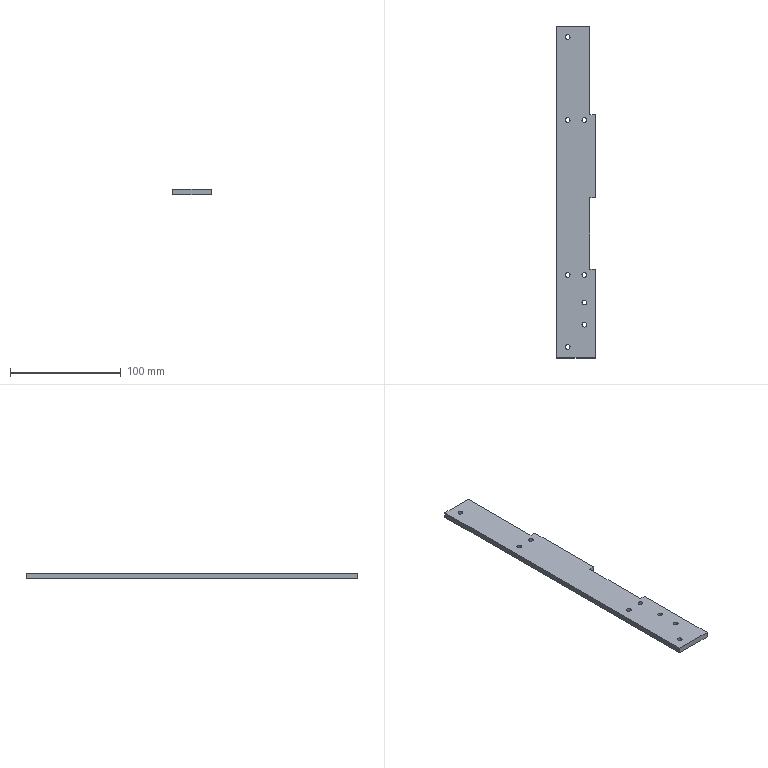Part | SolidWorks | features Extrusion 1 | 1 solid | 28 faces | box 35 x 300 x 5 mm | volume 48321 mm3 | cylinder 16 | plane 12 | commonest cylinder face diameters 4.2 x16
STEP:
#1=CARTESIAN_POINT('',(22.9,50.,5.));
#2=VERTEX_POINT('',#1);
#3=CARTESIAN_POINT('',(27.1,50.,5.));
#4=VERTEX_POINT('',#3);
#5=CARTESIAN_POINT('',(25.,50.,5.));
#6=DIRECTION('',(0.,0.,1.));
#7=DIRECTION('',(1.,0.,0.));
#8=AXIS2_PLACEMENT_3D('',#5,#6,#7);
#9=CIRCLE('',#8,2.1);
#10=EDGE_CURVE('',#2,#4,#9,.T.);
#11=ORIENTED_EDGE('',*,*,#10,.T.);
#12=CARTESIAN_POINT('',(27.1,50.,0.));
#13=VERTEX_POINT('',#12);
#14=CARTESIAN_POINT('',(27.1,50.,5.));
#15=DIRECTION('',(0.,0.,-1.));
#16=VECTOR('',#15,1000.);
#17=LINE('',#14,#16);
#18=EDGE_CURVE('',#4,#13,#17,.T.);
#19=ORIENTED_EDGE('',*,*,#18,.T.);
#20=CARTESIAN_POINT('',(22.9,50.,0.));
#21=VERTEX_POINT('',#20);
#22=CARTESIAN_POINT('',(25.,50.,0.));
#23=DIRECTION('',(0.,0.,1.));
#24=DIRECTION('',(1.,0.,0.));
#25=AXIS2_PLACEMENT_3D('',#22,#23,#24);
#26=CIRCLE('',#25,2.1);
#27=EDGE_CURVE('',#21,#13,#26,.T.);
#28=ORIENTED_EDGE('',*,*,#27,.F.);
#29=CARTESIAN_POINT('',(22.9,50.,5.));
#30=DIRECTION('',(0.,0.,-1.));
#31=VECTOR('',#30,1000.);
#32=LINE('',#29,#31);
#33=EDGE_CURVE('',#2,#21,#32,.T.);
#34=ORIENTED_EDGE('',*,*,#33,.F.);
#35=EDGE_LOOP('',(#11,#19,#28,#34));
#36=FACE_OUTER_BOUND('',#35,.T.);
#37=CARTESIAN_POINT('',(25.,50.,5.));
#38=DIRECTION('',(0.,0.,-1.));
#39=DIRECTION('',(-1.,0.,0.));
#40=AXIS2_PLACEMENT_3D('',#37,#38,#39);
#41=CYLINDRICAL_SURFACE('',#40,2.1);
#42=ADVANCED_FACE('',(#36),#41,.F.);
#43=CARTESIAN_POINT('',(22.9,30.,5.));
#44=VERTEX_POINT('',#43);
#45=CARTESIAN_POINT('',(27.1,30.,5.));
#46=VERTEX_POINT('',#45);
#47=CARTESIAN_POINT('',(25.,30.,5.));
#48=DIRECTION('',(0.,0.,1.));
#49=DIRECTION('',(1.,0.,0.));
#50=AXIS2_PLACEMENT_3D('',#47,#48,#49);
#51=CIRCLE('',#50,2.1);
#52=EDGE_CURVE('',#44,#46,#51,.T.);
#53=ORIENTED_EDGE('',*,*,#52,.T.);
#54=CARTESIAN_POINT('',(27.1,30.,0.));
#55=VERTEX_POINT('',#54);
#56=CARTESIAN_POINT('',(27.1,30.,5.));
#57=DIRECTION('',(0.,0.,-1.));
#58=VECTOR('',#57,1000.);
#59=LINE('',#56,#58);
#60=EDGE_CURVE('',#46,#55,#59,.T.);
#61=ORIENTED_EDGE('',*,*,#60,.T.);
#62=CARTESIAN_POINT('',(22.9,30.,0.));
#63=VERTEX_POINT('',#62);
#64=CARTESIAN_POINT('',(25.,30.,0.));
#65=DIRECTION('',(0.,0.,1.));
#66=DIRECTION('',(1.,0.,0.));
#67=AXIS2_PLACEMENT_3D('',#64,#65,#66);
#68=CIRCLE('',#67,2.1);
#69=EDGE_CURVE('',#63,#55,#68,.T.);
#70=ORIENTED_EDGE('',*,*,#69,.F.);
#71=CARTESIAN_POINT('',(22.9,30.,5.));
#72=DIRECTION('',(0.,0.,-1.));
#73=VECTOR('',#72,1000.);
#74=LINE('',#71,#73);
#75=EDGE_CURVE('',#44,#63,#74,.T.);
#76=ORIENTED_EDGE('',*,*,#75,.F.);
#77=EDGE_LOOP('',(#53,#61,#70,#76));
#78=FACE_OUTER_BOUND('',#77,.T.);
#79=CARTESIAN_POINT('',(25.,30.,5.));
#80=DIRECTION('',(0.,0.,-1.));
#81=DIRECTION('',(-1.,0.,0.));
#82=AXIS2_PLACEMENT_3D('',#79,#80,#81);
#83=CYLINDRICAL_SURFACE('',#82,2.1);
#84=ADVANCED_FACE('',(#78),#83,.F.);
#85=CARTESIAN_POINT('',(7.9,10.,5.));
#86=VERTEX_POINT('',#85);
#87=CARTESIAN_POINT('',(12.1,10.,5.));
#88=VERTEX_POINT('',#87);
#89=CARTESIAN_POINT('',(10.,10.,5.));
#90=DIRECTION('',(0.,0.,1.));
#91=DIRECTION('',(1.,0.,0.));
#92=AXIS2_PLACEMENT_3D('',#89,#90,#91);
#93=CIRCLE('',#92,2.1);
#94=EDGE_CURVE('',#86,#88,#93,.T.);
#95=ORIENTED_EDGE('',*,*,#94,.T.);
#96=CARTESIAN_POINT('',(12.1,10.,0.));
#97=VERTEX_POINT('',#96);
#98=CARTESIAN_POINT('',(12.1,10.,5.));
#99=DIRECTION('',(0.,0.,-1.));
#100=VECTOR('',#99,1000.);
#101=LINE('',#98,#100);
#102=EDGE_CURVE('',#88,#97,#101,.T.);
#103=ORIENTED_EDGE('',*,*,#102,.T.);
#104=CARTESIAN_POINT('',(7.9,10.,0.));
#105=VERTEX_POINT('',#104);
#106=CARTESIAN_POINT('',(10.,10.,0.));
#107=DIRECTION('',(0.,0.,1.));
#108=DIRECTION('',(1.,0.,0.));
#109=AXIS2_PLACEMENT_3D('',#106,#107,#108);
#110=CIRCLE('',#109,2.1);
#111=EDGE_CURVE('',#105,#97,#110,.T.);
#112=ORIENTED_EDGE('',*,*,#111,.F.);
#113=CARTESIAN_POINT('',(7.9,10.,5.));
#114=DIRECTION('',(0.,0.,-1.));
#115=VECTOR('',#114,1000.);
#116=LINE('',#113,#115);
#117=EDGE_CURVE('',#86,#105,#116,.T.);
#118=ORIENTED_EDGE('',*,*,#117,.F.);
#119=EDGE_LOOP('',(#95,#103,#112,#118));
#120=FACE_OUTER_BOUND('',#119,.T.);
#121=CARTESIAN_POINT('',(10.,10.,5.));
#122=DIRECTION('',(0.,0.,-1.));
#123=DIRECTION('',(-1.,0.,0.));
#124=AXIS2_PLACEMENT_3D('',#121,#122,#123);
#125=CYLINDRICAL_SURFACE('',#124,2.1);
#126=ADVANCED_FACE('',(#120),#125,.F.);
#127=CARTESIAN_POINT('',(7.9,290.,5.));
#128=VERTEX_POINT('',#127);
#129=CARTESIAN_POINT('',(12.1,290.,5.));
#130=VERTEX_POINT('',#129);
#131=CARTESIAN_POINT('',(10.,290.,5.));
#132=DIRECTION('',(0.,0.,1.));
#133=DIRECTION('',(1.,0.,0.));
#134=AXIS2_PLACEMENT_3D('',#131,#132,#133);
#135=CIRCLE('',#134,2.1);
#136=EDGE_CURVE('',#128,#130,#135,.T.);
#137=ORIENTED_EDGE('',*,*,#136,.T.);
#138=CARTESIAN_POINT('',(12.1,290.,0.));
#139=VERTEX_POINT('',#138);
#140=CARTESIAN_POINT('',(12.1,290.,5.));
#141=DIRECTION('',(0.,0.,-1.));
#142=VECTOR('',#141,1000.);
#143=LINE('',#140,#142);
#144=EDGE_CURVE('',#130,#139,#143,.T.);
#145=ORIENTED_EDGE('',*,*,#144,.T.);
#146=CARTESIAN_POINT('',(7.9,290.,0.));
#147=VERTEX_POINT('',#146);
#148=CARTESIAN_POINT('',(10.,290.,0.));
#149=DIRECTION('',(0.,0.,1.));
#150=DIRECTION('',(1.,0.,0.));
#151=AXIS2_PLACEMENT_3D('',#148,#149,#150);
#152=CIRCLE('',#151,2.1);
#153=EDGE_CURVE('',#147,#139,#152,.T.);
#154=ORIENTED_EDGE('',*,*,#153,.F.);
#155=CARTESIAN_POINT('',(7.9,290.,5.));
#156=DIRECTION('',(0.,0.,-1.));
#157=VECTOR('',#156,1000.);
#158=LINE('',#155,#157);
#159=EDGE_CURVE('',#128,#147,#158,.T.);
#160=ORIENTED_EDGE('',*,*,#159,.F.);
#161=EDGE_LOOP('',(#137,#145,#154,#160));
#162=FACE_OUTER_BOUND('',#161,.T.);
#163=CARTESIAN_POINT('',(10.,290.,5.));
#164=DIRECTION('',(0.,0.,-1.));
#165=DIRECTION('',(-1.,0.,0.));
#166=AXIS2_PLACEMENT_3D('',#163,#164,#165);
#167=CYLINDRICAL_SURFACE('',#166,2.1);
#168=ADVANCED_FACE('',(#162),#167,.F.);
#169=CARTESIAN_POINT('',(7.9,75.,5.));
#170=VERTEX_POINT('',#169);
#171=CARTESIAN_POINT('',(12.1,75.,5.));
#172=VERTEX_POINT('',#171);
#173=CARTESIAN_POINT('',(10.,75.,5.));
#174=DIRECTION('',(0.,0.,1.));
#175=DIRECTION('',(1.,0.,0.));
#176=AXIS2_PLACEMENT_3D('',#173,#174,#175);
#177=CIRCLE('',#176,2.1);
#178=EDGE_CURVE('',#170,#172,#177,.T.);
#179=ORIENTED_EDGE('',*,*,#178,.T.);
#180=CARTESIAN_POINT('',(12.1,75.,0.));
#181=VERTEX_POINT('',#180);
#182=CARTESIAN_POINT('',(12.1,75.,5.));
#183=DIRECTION('',(0.,0.,-1.));
#184=VECTOR('',#183,1000.);
#185=LINE('',#182,#184);
#186=EDGE_CURVE('',#172,#181,#185,.T.);
#187=ORIENTED_EDGE('',*,*,#186,.T.);
#188=CARTESIAN_POINT('',(7.9,75.,0.));
#189=VERTEX_POINT('',#188);
#190=CARTESIAN_POINT('',(10.,75.,0.));
#191=DIRECTION('',(0.,0.,1.));
#192=DIRECTION('',(1.,0.,0.));
#193=AXIS2_PLACEMENT_3D('',#190,#191,#192);
#194=CIRCLE('',#193,2.1);
#195=EDGE_CURVE('',#189,#181,#194,.T.);
#196=ORIENTED_EDGE('',*,*,#195,.F.);
#197=CARTESIAN_POINT('',(7.9,75.,5.));
#198=DIRECTION('',(0.,0.,-1.));
#199=VECTOR('',#198,1000.);
#200=LINE('',#197,#199);
#201=EDGE_CURVE('',#170,#189,#200,.T.);
#202=ORIENTED_EDGE('',*,*,#201,.F.);
#203=EDGE_LOOP('',(#179,#187,#196,#202));
#204=FACE_OUTER_BOUND('',#203,.T.);
#205=CARTESIAN_POINT('',(10.,75.,5.));
#206=DIRECTION('',(0.,0.,-1.));
#207=DIRECTION('',(-1.,0.,0.));
#208=AXIS2_PLACEMENT_3D('',#205,#206,#207);
#209=CYLINDRICAL_SURFACE('',#208,2.1);
#210=ADVANCED_FACE('',(#204),#209,.F.);
#211=CARTESIAN_POINT('',(22.9,75.,5.));
#212=VERTEX_POINT('',#211);
#213=CARTESIAN_POINT('',(27.1,75.,5.));
#214=VERTEX_POINT('',#213);
#215=CARTESIAN_POINT('',(25.,75.,5.));
#216=DIRECTION('',(0.,0.,1.));
#217=DIRECTION('',(1.,0.,0.));
#218=AXIS2_PLACEMENT_3D('',#215,#216,#217);
#219=CIRCLE('',#218,2.1);
#220=EDGE_CURVE('',#212,#214,#219,.T.);
#221=ORIENTED_EDGE('',*,*,#220,.T.);
#222=CARTESIAN_POINT('',(27.1,75.,0.));
#223=VERTEX_POINT('',#222);
#224=CARTESIAN_POINT('',(27.1,75.,5.));
#225=DIRECTION('',(0.,0.,-1.));
#226=VECTOR('',#225,1000.);
#227=LINE('',#224,#226);
#228=EDGE_CURVE('',#214,#223,#227,.T.);
#229=ORIENTED_EDGE('',*,*,#228,.T.);
#230=CARTESIAN_POINT('',(22.9,75.,0.));
#231=VERTEX_POINT('',#230);
#232=CARTESIAN_POINT('',(25.,75.,0.));
#233=DIRECTION('',(0.,0.,1.));
#234=DIRECTION('',(1.,0.,0.));
#235=AXIS2_PLACEMENT_3D('',#232,#233,#234);
#236=CIRCLE('',#235,2.1);
#237=EDGE_CURVE('',#231,#223,#236,.T.);
#238=ORIENTED_EDGE('',*,*,#237,.F.);
#239=CARTESIAN_POINT('',(22.9,75.,5.));
#240=DIRECTION('',(0.,0.,-1.));
#241=VECTOR('',#240,1000.);
#242=LINE('',#239,#241);
#243=EDGE_CURVE('',#212,#231,#242,.T.);
#244=ORIENTED_EDGE('',*,*,#243,.F.);
#245=EDGE_LOOP('',(#221,#229,#238,#244));
#246=FACE_OUTER_BOUND('',#245,.T.);
#247=CARTESIAN_POINT('',(25.,75.,5.));
#248=DIRECTION('',(0.,0.,-1.));
#249=DIRECTION('',(-1.,0.,0.));
#250=AXIS2_PLACEMENT_3D('',#247,#248,#249);
#251=CYLINDRICAL_SURFACE('',#250,2.1);
#252=ADVANCED_FACE('',(#246),#251,.F.);
#253=CARTESIAN_POINT('',(7.9,215.,5.));
#254=VERTEX_POINT('',#253);
#255=CARTESIAN_POINT('',(12.1,215.,5.));
#256=VERTEX_POINT('',#255);
#257=CARTESIAN_POINT('',(10.,215.,5.));
#258=DIRECTION('',(0.,0.,1.));
#259=DIRECTION('',(1.,0.,0.));
#260=AXIS2_PLACEMENT_3D('',#257,#258,#259);
#261=CIRCLE('',#260,2.1);
#262=EDGE_CURVE('',#254,#256,#261,.T.);
#263=ORIENTED_EDGE('',*,*,#262,.T.);
#264=CARTESIAN_POINT('',(12.1,215.,0.));
#265=VERTEX_POINT('',#264);
#266=CARTESIAN_POINT('',(12.1,215.,5.));
#267=DIRECTION('',(0.,0.,-1.));
#268=VECTOR('',#267,1000.);
#269=LINE('',#266,#268);
#270=EDGE_CURVE('',#256,#265,#269,.T.);
#271=ORIENTED_EDGE('',*,*,#270,.T.);
#272=CARTESIAN_POINT('',(7.9,215.,0.));
#273=VERTEX_POINT('',#272);
#274=CARTESIAN_POINT('',(10.,215.,0.));
#275=DIRECTION('',(0.,0.,1.));
#276=DIRECTION('',(1.,0.,0.));
#277=AXIS2_PLACEMENT_3D('',#274,#275,#276);
#278=CIRCLE('',#277,2.1);
#279=EDGE_CURVE('',#273,#265,#278,.T.);
#280=ORIENTED_EDGE('',*,*,#279,.F.);
#281=CARTESIAN_POINT('',(7.9,215.,5.));
#282=DIRECTION('',(0.,0.,-1.));
#283=VECTOR('',#282,1000.);
#284=LINE('',#281,#283);
#285=EDGE_CURVE('',#254,#273,#284,.T.);
#286=ORIENTED_EDGE('',*,*,#285,.F.);
#287=EDGE_LOOP('',(#263,#271,#280,#286));
#288=FACE_OUTER_BOUND('',#287,.T.);
#289=CARTESIAN_POINT('',(10.,215.,5.));
#290=DIRECTION('',(0.,0.,-1.));
#291=DIRECTION('',(-1.,0.,0.));
#292=AXIS2_PLACEMENT_3D('',#289,#290,#291);
#293=CYLINDRICAL_SURFACE('',#292,2.1);
#294=ADVANCED_FACE('',(#288),#293,.F.);
#295=CARTESIAN_POINT('',(22.9,215.,5.));
#296=VERTEX_POINT('',#295);
#297=CARTESIAN_POINT('',(27.1,215.,5.));
#298=VERTEX_POINT('',#297);
#299=CARTESIAN_POINT('',(25.,215.,5.));
#300=DIRECTION('',(0.,0.,1.));
#301=DIRECTION('',(1.,0.,0.));
#302=AXIS2_PLACEMENT_3D('',#299,#300,#301);
#303=CIRCLE('',#302,2.1);
#304=EDGE_CURVE('',#296,#298,#303,.T.);
#305=ORIENTED_EDGE('',*,*,#304,.T.);
#306=CARTESIAN_POINT('',(27.1,215.,0.));
#307=VERTEX_POINT('',#306);
#308=CARTESIAN_POINT('',(27.1,215.,5.));
#309=DIRECTION('',(0.,0.,-1.));
#310=VECTOR('',#309,1000.);
#311=LINE('',#308,#310);
#312=EDGE_CURVE('',#298,#307,#311,.T.);
#313=ORIENTED_EDGE('',*,*,#312,.T.);
#314=CARTESIAN_POINT('',(22.9,215.,0.));
#315=VERTEX_POINT('',#314);
#316=CARTESIAN_POINT('',(25.,215.,0.));
#317=DIRECTION('',(0.,0.,1.));
#318=DIRECTION('',(1.,0.,0.));
#319=AXIS2_PLACEMENT_3D('',#316,#317,#318);
#320=CIRCLE('',#319,2.1);
#321=EDGE_CURVE('',#315,#307,#320,.T.);
#322=ORIENTED_EDGE('',*,*,#321,.F.);
#323=CARTESIAN_POINT('',(22.9,215.,5.));
#324=DIRECTION('',(0.,0.,-1.));
#325=VECTOR('',#324,1000.);
#326=LINE('',#323,#325);
#327=EDGE_CURVE('',#296,#315,#326,.T.);
#328=ORIENTED_EDGE('',*,*,#327,.F.);
#329=EDGE_LOOP('',(#305,#313,#322,#328));
#330=FACE_OUTER_BOUND('',#329,.T.);
#331=CARTESIAN_POINT('',(25.,215.,5.));
#332=DIRECTION('',(0.,0.,-1.));
#333=DIRECTION('',(-1.,0.,0.));
#334=AXIS2_PLACEMENT_3D('',#331,#332,#333);
#335=CYLINDRICAL_SURFACE('',#334,2.1);
#336=ADVANCED_FACE('',(#330),#335,.F.);
#337=CARTESIAN_POINT('',(0.,300.,5.));
#338=VERTEX_POINT('',#337);
#339=CARTESIAN_POINT('',(0.,0.,5.));
#340=VERTEX_POINT('',#339);
#341=CARTESIAN_POINT('',(0.,0.,5.));
#342=DIRECTION('',(0.,-1.,0.));
#343=VECTOR('',#342,1000.);
#344=LINE('',#341,#343);
#345=EDGE_CURVE('',#338,#340,#344,.T.);
#346=ORIENTED_EDGE('',*,*,#345,.T.);
#347=CARTESIAN_POINT('',(35.,0.,5.));
#348=VERTEX_POINT('',#347);
#349=CARTESIAN_POINT('',(0.,0.,5.));
#350=DIRECTION('',(1.,0.,0.));
#351=VECTOR('',#350,1000.);
#352=LINE('',#349,#351);
#353=EDGE_CURVE('',#340,#348,#352,.T.);
#354=ORIENTED_EDGE('',*,*,#353,.T.);
#355=CARTESIAN_POINT('',(35.,80.,5.));
#356=VERTEX_POINT('',#355);
#357=CARTESIAN_POINT('',(35.,0.,5.));
#358=DIRECTION('',(0.,1.,0.));
#359=VECTOR('',#358,1000.);
#360=LINE('',#357,#359);
#361=EDGE_CURVE('',#348,#356,#360,.T.);
#362=ORIENTED_EDGE('',*,*,#361,.T.);
#363=CARTESIAN_POINT('',(30.,80.,5.));
#364=VERTEX_POINT('',#363);
#365=CARTESIAN_POINT('',(30.,80.,5.));
#366=DIRECTION('',(-1.,0.,0.));
#367=VECTOR('',#366,1000.);
#368=LINE('',#365,#367);
#369=EDGE_CURVE('',#356,#364,#368,.T.);
#370=ORIENTED_EDGE('',*,*,#369,.T.);
#371=CARTESIAN_POINT('',(30.,145.,5.));
#372=VERTEX_POINT('',#371);
#373=CARTESIAN_POINT('',(30.,145.,5.));
#374=DIRECTION('',(0.,1.,0.));
#375=VECTOR('',#374,1000.);
#376=LINE('',#373,#375);
#377=EDGE_CURVE('',#364,#372,#376,.T.);
#378=ORIENTED_EDGE('',*,*,#377,.T.);
#379=CARTESIAN_POINT('',(35.,145.,5.));
#380=VERTEX_POINT('',#379);
#381=CARTESIAN_POINT('',(35.,145.,5.));
#382=DIRECTION('',(1.,0.,0.));
#383=VECTOR('',#382,1000.);
#384=LINE('',#381,#383);
#385=EDGE_CURVE('',#372,#380,#384,.T.);
#386=ORIENTED_EDGE('',*,*,#385,.T.);
#387=CARTESIAN_POINT('',(35.,220.,5.));
#388=VERTEX_POINT('',#387);
#389=CARTESIAN_POINT('',(35.,145.,5.));
#390=DIRECTION('',(0.,1.,0.));
#391=VECTOR('',#390,1000.);
#392=LINE('',#389,#391);
#393=EDGE_CURVE('',#380,#388,#392,.T.);
#394=ORIENTED_EDGE('',*,*,#393,.T.);
#395=CARTESIAN_POINT('',(30.,220.,5.));
#396=VERTEX_POINT('',#395);
#397=CARTESIAN_POINT('',(30.,220.,5.));
#398=DIRECTION('',(-1.,0.,0.));
#399=VECTOR('',#398,1000.);
#400=LINE('',#397,#399);
#401=EDGE_CURVE('',#388,#396,#400,.T.);
#402=ORIENTED_EDGE('',*,*,#401,.T.);
#403=CARTESIAN_POINT('',(30.,300.,5.));
#404=VERTEX_POINT('',#403);
#405=CARTESIAN_POINT('',(30.,300.,5.));
#406=DIRECTION('',(0.,1.,0.));
#407=VECTOR('',#406,1000.);
#408=LINE('',#405,#407);
#409=EDGE_CURVE('',#396,#404,#408,.T.);
#410=ORIENTED_EDGE('',*,*,#409,.T.);
#411=CARTESIAN_POINT('',(0.,300.,5.));
#412=DIRECTION('',(-1.,0.,0.));
#413=VECTOR('',#412,1000.);
#414=LINE('',#411,#413);
#415=EDGE_CURVE('',#404,#338,#414,.T.);
#416=ORIENTED_EDGE('',*,*,#415,.T.);
#417=EDGE_LOOP('',(#346,#354,#362,#370,#378,#386,#394,#402,#410,#416));
#418=FACE_OUTER_BOUND('',#417,.T.);
#419=ORIENTED_EDGE('',*,*,#304,.F.);
#420=CARTESIAN_POINT('',(25.,215.,5.));
#421=DIRECTION('',(0.,0.,1.));
#422=DIRECTION('',(1.,0.,0.));
#423=AXIS2_PLACEMENT_3D('',#420,#421,#422);
#424=CIRCLE('',#423,2.1);
#425=EDGE_CURVE('',#298,#296,#424,.T.);
#426=ORIENTED_EDGE('',*,*,#425,.F.);
#427=EDGE_LOOP('',(#419,#426));
#428=FACE_BOUND('',#427,.T.);
#429=ORIENTED_EDGE('',*,*,#262,.F.);
#430=CARTESIAN_POINT('',(10.,215.,5.));
#431=DIRECTION('',(0.,0.,1.));
#432=DIRECTION('',(1.,0.,0.));
#433=AXIS2_PLACEMENT_3D('',#430,#431,#432);
#434=CIRCLE('',#433,2.1);
#435=EDGE_CURVE('',#256,#254,#434,.T.);
#436=ORIENTED_EDGE('',*,*,#435,.F.);
#437=EDGE_LOOP('',(#429,#436));
#438=FACE_BOUND('',#437,.T.);
#439=ORIENTED_EDGE('',*,*,#220,.F.);
#440=CARTESIAN_POINT('',(25.,75.,5.));
#441=DIRECTION('',(0.,0.,1.));
#442=DIRECTION('',(1.,0.,0.));
#443=AXIS2_PLACEMENT_3D('',#440,#441,#442);
#444=CIRCLE('',#443,2.1);
#445=EDGE_CURVE('',#214,#212,#444,.T.);
#446=ORIENTED_EDGE('',*,*,#445,.F.);
#447=EDGE_LOOP('',(#439,#446));
#448=FACE_BOUND('',#447,.T.);
#449=ORIENTED_EDGE('',*,*,#178,.F.);
#450=CARTESIAN_POINT('',(10.,75.,5.));
#451=DIRECTION('',(0.,0.,1.));
#452=DIRECTION('',(1.,0.,0.));
#453=AXIS2_PLACEMENT_3D('',#450,#451,#452);
#454=CIRCLE('',#453,2.1);
#455=EDGE_CURVE('',#172,#170,#454,.T.);
#456=ORIENTED_EDGE('',*,*,#455,.F.);
#457=EDGE_LOOP('',(#449,#456));
#458=FACE_BOUND('',#457,.T.);
#459=ORIENTED_EDGE('',*,*,#136,.F.);
#460=CARTESIAN_POINT('',(10.,290.,5.));
#461=DIRECTION('',(0.,0.,1.));
#462=DIRECTION('',(1.,0.,0.));
#463=AXIS2_PLACEMENT_3D('',#460,#461,#462);
#464=CIRCLE('',#463,2.1);
#465=EDGE_CURVE('',#130,#128,#464,.T.);
#466=ORIENTED_EDGE('',*,*,#465,.F.);
#467=EDGE_LOOP('',(#459,#466));
#468=FACE_BOUND('',#467,.T.);
#469=ORIENTED_EDGE('',*,*,#94,.F.);
#470=CARTESIAN_POINT('',(10.,10.,5.));
#471=DIRECTION('',(0.,0.,1.));
#472=DIRECTION('',(1.,0.,0.));
#473=AXIS2_PLACEMENT_3D('',#470,#471,#472);
#474=CIRCLE('',#473,2.1);
#475=EDGE_CURVE('',#88,#86,#474,.T.);
#476=ORIENTED_EDGE('',*,*,#475,.F.);
#477=EDGE_LOOP('',(#469,#476));
#478=FACE_BOUND('',#477,.T.);
#479=ORIENTED_EDGE('',*,*,#52,.F.);
#480=CARTESIAN_POINT('',(25.,30.,5.));
#481=DIRECTION('',(0.,0.,1.));
#482=DIRECTION('',(1.,0.,0.));
#483=AXIS2_PLACEMENT_3D('',#480,#481,#482);
#484=CIRCLE('',#483,2.1);
#485=EDGE_CURVE('',#46,#44,#484,.T.);
#486=ORIENTED_EDGE('',*,*,#485,.F.);
#487=EDGE_LOOP('',(#479,#486));
#488=FACE_BOUND('',#487,.T.);
#489=ORIENTED_EDGE('',*,*,#10,.F.);
#490=CARTESIAN_POINT('',(25.,50.,5.));
#491=DIRECTION('',(0.,0.,1.));
#492=DIRECTION('',(1.,0.,0.));
#493=AXIS2_PLACEMENT_3D('',#490,#491,#492);
#494=CIRCLE('',#493,2.1);
#495=EDGE_CURVE('',#4,#2,#494,.T.);
#496=ORIENTED_EDGE('',*,*,#495,.F.);
#497=EDGE_LOOP('',(#489,#496));
#498=FACE_BOUND('',#497,.T.);
#499=CARTESIAN_POINT('',(0.,0.,5.));
#500=DIRECTION('',(0.,0.,-1.));
#501=DIRECTION('',(-1.,0.,0.));
#502=AXIS2_PLACEMENT_3D('',#499,#500,#501);
#503=PLANE('',#502);
#504=ADVANCED_FACE('',(#418,#428,#438,#448,#458,#468,#478,#488,#498),#503,.F.);
#505=ORIENTED_EDGE('',*,*,#69,.T.);
#506=CARTESIAN_POINT('',(25.,30.,0.));
#507=DIRECTION('',(0.,0.,1.));
#508=DIRECTION('',(1.,0.,0.));
#509=AXIS2_PLACEMENT_3D('',#506,#507,#508);
#510=CIRCLE('',#509,2.1);
#511=EDGE_CURVE('',#55,#63,#510,.T.);
#512=ORIENTED_EDGE('',*,*,#511,.T.);
#513=EDGE_LOOP('',(#505,#512));
#514=FACE_BOUND('',#513,.T.);
#515=ORIENTED_EDGE('',*,*,#153,.T.);
#516=CARTESIAN_POINT('',(10.,290.,0.));
#517=DIRECTION('',(0.,0.,1.));
#518=DIRECTION('',(1.,0.,0.));
#519=AXIS2_PLACEMENT_3D('',#516,#517,#518);
#520=CIRCLE('',#519,2.1);
#521=EDGE_CURVE('',#139,#147,#520,.T.);
#522=ORIENTED_EDGE('',*,*,#521,.T.);
#523=EDGE_LOOP('',(#515,#522));
#524=FACE_BOUND('',#523,.T.);
#525=ORIENTED_EDGE('',*,*,#237,.T.);
#526=CARTESIAN_POINT('',(25.,75.,0.));
#527=DIRECTION('',(0.,0.,1.));
#528=DIRECTION('',(1.,0.,0.));
#529=AXIS2_PLACEMENT_3D('',#526,#527,#528);
#530=CIRCLE('',#529,2.1);
#531=EDGE_CURVE('',#223,#231,#530,.T.);
#532=ORIENTED_EDGE('',*,*,#531,.T.);
#533=EDGE_LOOP('',(#525,#532));
#534=FACE_BOUND('',#533,.T.);
#535=ORIENTED_EDGE('',*,*,#321,.T.);
#536=CARTESIAN_POINT('',(25.,215.,0.));
#537=DIRECTION('',(0.,0.,1.));
#538=DIRECTION('',(1.,0.,0.));
#539=AXIS2_PLACEMENT_3D('',#536,#537,#538);
#540=CIRCLE('',#539,2.1);
#541=EDGE_CURVE('',#307,#315,#540,.T.);
#542=ORIENTED_EDGE('',*,*,#541,.T.);
#543=EDGE_LOOP('',(#535,#542));
#544=FACE_BOUND('',#543,.T.);
#545=CARTESIAN_POINT('',(0.,300.,0.));
#546=VERTEX_POINT('',#545);
#547=CARTESIAN_POINT('',(0.,0.,0.));
#548=VERTEX_POINT('',#547);
#549=CARTESIAN_POINT('',(0.,0.,0.));
#550=DIRECTION('',(0.,-1.,0.));
#551=VECTOR('',#550,1000.);
#552=LINE('',#549,#551);
#553=EDGE_CURVE('',#546,#548,#552,.T.);
#554=ORIENTED_EDGE('',*,*,#553,.F.);
#555=CARTESIAN_POINT('',(30.,300.,0.));
#556=VERTEX_POINT('',#555);
#557=CARTESIAN_POINT('',(0.,300.,0.));
#558=DIRECTION('',(-1.,0.,0.));
#559=VECTOR('',#558,1000.);
#560=LINE('',#557,#559);
#561=EDGE_CURVE('',#556,#546,#560,.T.);
#562=ORIENTED_EDGE('',*,*,#561,.F.);
#563=CARTESIAN_POINT('',(30.,220.,0.));
#564=VERTEX_POINT('',#563);
#565=CARTESIAN_POINT('',(30.,300.,0.));
#566=DIRECTION('',(0.,1.,0.));
#567=VECTOR('',#566,1000.);
#568=LINE('',#565,#567);
#569=EDGE_CURVE('',#564,#556,#568,.T.);
#570=ORIENTED_EDGE('',*,*,#569,.F.);
#571=CARTESIAN_POINT('',(35.,220.,0.));
#572=VERTEX_POINT('',#571);
#573=CARTESIAN_POINT('',(30.,220.,0.));
#574=DIRECTION('',(-1.,0.,0.));
#575=VECTOR('',#574,1000.);
#576=LINE('',#573,#575);
#577=EDGE_CURVE('',#572,#564,#576,.T.);
#578=ORIENTED_EDGE('',*,*,#577,.F.);
#579=CARTESIAN_POINT('',(35.,145.,0.));
#580=VERTEX_POINT('',#579);
#581=CARTESIAN_POINT('',(35.,145.,0.));
#582=DIRECTION('',(0.,1.,0.));
#583=VECTOR('',#582,1000.);
#584=LINE('',#581,#583);
#585=EDGE_CURVE('',#580,#572,#584,.T.);
#586=ORIENTED_EDGE('',*,*,#585,.F.);
#587=CARTESIAN_POINT('',(30.,145.,0.));
#588=VERTEX_POINT('',#587);
#589=CARTESIAN_POINT('',(35.,145.,0.));
#590=DIRECTION('',(1.,0.,0.));
#591=VECTOR('',#590,1000.);
#592=LINE('',#589,#591);
#593=EDGE_CURVE('',#588,#580,#592,.T.);
#594=ORIENTED_EDGE('',*,*,#593,.F.);
#595=CARTESIAN_POINT('',(30.,80.,0.));
#596=VERTEX_POINT('',#595);
#597=CARTESIAN_POINT('',(30.,145.,0.));
#598=DIRECTION('',(0.,1.,0.));
#599=VECTOR('',#598,1000.);
#600=LINE('',#597,#599);
#601=EDGE_CURVE('',#596,#588,#600,.T.);
#602=ORIENTED_EDGE('',*,*,#601,.F.);
#603=CARTESIAN_POINT('',(35.,80.,0.));
#604=VERTEX_POINT('',#603);
#605=CARTESIAN_POINT('',(30.,80.,0.));
#606=DIRECTION('',(-1.,0.,0.));
#607=VECTOR('',#606,1000.);
#608=LINE('',#605,#607);
#609=EDGE_CURVE('',#604,#596,#608,.T.);
#610=ORIENTED_EDGE('',*,*,#609,.F.);
#611=CARTESIAN_POINT('',(35.,0.,0.));
#612=VERTEX_POINT('',#611);
#613=CARTESIAN_POINT('',(35.,0.,0.));
#614=DIRECTION('',(0.,1.,0.));
#615=VECTOR('',#614,1000.);
#616=LINE('',#613,#615);
#617=EDGE_CURVE('',#612,#604,#616,.T.);
#618=ORIENTED_EDGE('',*,*,#617,.F.);
#619=CARTESIAN_POINT('',(0.,0.,0.));
#620=DIRECTION('',(1.,0.,0.));
#621=VECTOR('',#620,1000.);
#622=LINE('',#619,#621);
#623=EDGE_CURVE('',#548,#612,#622,.T.);
#624=ORIENTED_EDGE('',*,*,#623,.F.);
#625=EDGE_LOOP('',(#554,#562,#570,#578,#586,#594,#602,#610,#618,#624));
#626=FACE_OUTER_BOUND('',#625,.T.);
#627=ORIENTED_EDGE('',*,*,#279,.T.);
#628=CARTESIAN_POINT('',(10.,215.,0.));
#629=DIRECTION('',(0.,0.,1.));
#630=DIRECTION('',(1.,0.,0.));
#631=AXIS2_PLACEMENT_3D('',#628,#629,#630);
#632=CIRCLE('',#631,2.1);
#633=EDGE_CURVE('',#265,#273,#632,.T.);
#634=ORIENTED_EDGE('',*,*,#633,.T.);
#635=EDGE_LOOP('',(#627,#634));
#636=FACE_BOUND('',#635,.T.);
#637=ORIENTED_EDGE('',*,*,#195,.T.);
#638=CARTESIAN_POINT('',(10.,75.,0.));
#639=DIRECTION('',(0.,0.,1.));
#640=DIRECTION('',(1.,0.,0.));
#641=AXIS2_PLACEMENT_3D('',#638,#639,#640);
#642=CIRCLE('',#641,2.1);
#643=EDGE_CURVE('',#181,#189,#642,.T.);
#644=ORIENTED_EDGE('',*,*,#643,.T.);
#645=EDGE_LOOP('',(#637,#644));
#646=FACE_BOUND('',#645,.T.);
#647=ORIENTED_EDGE('',*,*,#111,.T.);
#648=CARTESIAN_POINT('',(10.,10.,0.));
#649=DIRECTION('',(0.,0.,1.));
#650=DIRECTION('',(1.,0.,0.));
#651=AXIS2_PLACEMENT_3D('',#648,#649,#650);
#652=CIRCLE('',#651,2.1);
#653=EDGE_CURVE('',#97,#105,#652,.T.);
#654=ORIENTED_EDGE('',*,*,#653,.T.);
#655=EDGE_LOOP('',(#647,#654));
#656=FACE_BOUND('',#655,.T.);
#657=ORIENTED_EDGE('',*,*,#27,.T.);
#658=CARTESIAN_POINT('',(25.,50.,0.));
#659=DIRECTION('',(0.,0.,1.));
#660=DIRECTION('',(1.,0.,0.));
#661=AXIS2_PLACEMENT_3D('',#658,#659,#660);
#662=CIRCLE('',#661,2.1);
#663=EDGE_CURVE('',#13,#21,#662,.T.);
#664=ORIENTED_EDGE('',*,*,#663,.T.);
#665=EDGE_LOOP('',(#657,#664));
#666=FACE_BOUND('',#665,.T.);
#667=CARTESIAN_POINT('',(0.,0.,0.));
#668=DIRECTION('',(0.,0.,-1.));
#669=DIRECTION('',(-1.,0.,0.));
#670=AXIS2_PLACEMENT_3D('',#667,#668,#669);
#671=PLANE('',#670);
#672=ADVANCED_FACE('',(#514,#524,#534,#544,#626,#636,#646,#656,#666),#671,.T.);
#673=ORIENTED_EDGE('',*,*,#553,.T.);
#674=CARTESIAN_POINT('',(0.,0.,5.));
#675=DIRECTION('',(0.,0.,-1.));
#676=VECTOR('',#675,1000.);
#677=LINE('',#674,#676);
#678=EDGE_CURVE('',#340,#548,#677,.T.);
#679=ORIENTED_EDGE('',*,*,#678,.F.);
#680=ORIENTED_EDGE('',*,*,#345,.F.);
#681=CARTESIAN_POINT('',(0.,300.,5.));
#682=DIRECTION('',(0.,0.,-1.));
#683=VECTOR('',#682,1000.);
#684=LINE('',#681,#683);
#685=EDGE_CURVE('',#338,#546,#684,.T.);
#686=ORIENTED_EDGE('',*,*,#685,.T.);
#687=EDGE_LOOP('',(#673,#679,#680,#686));
#688=FACE_OUTER_BOUND('',#687,.T.);
#689=CARTESIAN_POINT('',(0.,0.,5.));
#690=DIRECTION('',(1.,0.,0.));
#691=DIRECTION('',(0.,0.,-1.));
#692=AXIS2_PLACEMENT_3D('',#689,#690,#691);
#693=PLANE('',#692);
#694=ADVANCED_FACE('',(#688),#693,.F.);
#695=ORIENTED_EDGE('',*,*,#623,.T.);
#696=CARTESIAN_POINT('',(35.,0.,5.));
#697=DIRECTION('',(0.,0.,-1.));
#698=VECTOR('',#697,1000.);
#699=LINE('',#696,#698);
#700=EDGE_CURVE('',#348,#612,#699,.T.);
#701=ORIENTED_EDGE('',*,*,#700,.F.);
#702=ORIENTED_EDGE('',*,*,#353,.F.);
#703=ORIENTED_EDGE('',*,*,#678,.T.);
#704=EDGE_LOOP('',(#695,#701,#702,#703));
#705=FACE_OUTER_BOUND('',#704,.T.);
#706=CARTESIAN_POINT('',(0.,0.,5.));
#707=DIRECTION('',(0.,1.,0.));
#708=DIRECTION('',(0.,0.,1.));
#709=AXIS2_PLACEMENT_3D('',#706,#707,#708);
#710=PLANE('',#709);
#711=ADVANCED_FACE('',(#705),#710,.F.);
#712=ORIENTED_EDGE('',*,*,#617,.T.);
#713=CARTESIAN_POINT('',(35.,80.,5.));
#714=DIRECTION('',(0.,0.,-1.));
#715=VECTOR('',#714,1000.);
#716=LINE('',#713,#715);
#717=EDGE_CURVE('',#356,#604,#716,.T.);
#718=ORIENTED_EDGE('',*,*,#717,.F.);
#719=ORIENTED_EDGE('',*,*,#361,.F.);
#720=ORIENTED_EDGE('',*,*,#700,.T.);
#721=EDGE_LOOP('',(#712,#718,#719,#720));
#722=FACE_OUTER_BOUND('',#721,.T.);
#723=CARTESIAN_POINT('',(35.,0.,5.));
#724=DIRECTION('',(-1.,0.,0.));
#725=DIRECTION('',(0.,-1.,0.));
#726=AXIS2_PLACEMENT_3D('',#723,#724,#725);
#727=PLANE('',#726);
#728=ADVANCED_FACE('',(#722),#727,.F.);
#729=ORIENTED_EDGE('',*,*,#609,.T.);
#730=CARTESIAN_POINT('',(30.,80.,5.));
#731=DIRECTION('',(0.,0.,-1.));
#732=VECTOR('',#731,1000.);
#733=LINE('',#730,#732);
#734=EDGE_CURVE('',#364,#596,#733,.T.);
#735=ORIENTED_EDGE('',*,*,#734,.F.);
#736=ORIENTED_EDGE('',*,*,#369,.F.);
#737=ORIENTED_EDGE('',*,*,#717,.T.);
#738=EDGE_LOOP('',(#729,#735,#736,#737));
#739=FACE_OUTER_BOUND('',#738,.T.);
#740=CARTESIAN_POINT('',(30.,80.,5.));
#741=DIRECTION('',(0.,-1.,0.));
#742=DIRECTION('',(0.,0.,-1.));
#743=AXIS2_PLACEMENT_3D('',#740,#741,#742);
#744=PLANE('',#743);
#745=ADVANCED_FACE('',(#739),#744,.F.);
#746=ORIENTED_EDGE('',*,*,#601,.T.);
#747=CARTESIAN_POINT('',(30.,145.,5.));
#748=DIRECTION('',(0.,0.,-1.));
#749=VECTOR('',#748,1000.);
#750=LINE('',#747,#749);
#751=EDGE_CURVE('',#372,#588,#750,.T.);
#752=ORIENTED_EDGE('',*,*,#751,.F.);
#753=ORIENTED_EDGE('',*,*,#377,.F.);
#754=ORIENTED_EDGE('',*,*,#734,.T.);
#755=EDGE_LOOP('',(#746,#752,#753,#754));
#756=FACE_OUTER_BOUND('',#755,.T.);
#757=CARTESIAN_POINT('',(30.,145.,5.));
#758=DIRECTION('',(-1.,0.,0.));
#759=DIRECTION('',(0.,-1.,0.));
#760=AXIS2_PLACEMENT_3D('',#757,#758,#759);
#761=PLANE('',#760);
#762=ADVANCED_FACE('',(#756),#761,.F.);
#763=ORIENTED_EDGE('',*,*,#593,.T.);
#764=CARTESIAN_POINT('',(35.,145.,5.));
#765=DIRECTION('',(0.,0.,-1.));
#766=VECTOR('',#765,1000.);
#767=LINE('',#764,#766);
#768=EDGE_CURVE('',#380,#580,#767,.T.);
#769=ORIENTED_EDGE('',*,*,#768,.F.);
#770=ORIENTED_EDGE('',*,*,#385,.F.);
#771=ORIENTED_EDGE('',*,*,#751,.T.);
#772=EDGE_LOOP('',(#763,#769,#770,#771));
#773=FACE_OUTER_BOUND('',#772,.T.);
#774=CARTESIAN_POINT('',(35.,145.,5.));
#775=DIRECTION('',(0.,1.,0.));
#776=DIRECTION('',(0.,0.,1.));
#777=AXIS2_PLACEMENT_3D('',#774,#775,#776);
#778=PLANE('',#777);
#779=ADVANCED_FACE('',(#773),#778,.F.);
#780=ORIENTED_EDGE('',*,*,#585,.T.);
#781=CARTESIAN_POINT('',(35.,220.,5.));
#782=DIRECTION('',(0.,0.,-1.));
#783=VECTOR('',#782,1000.);
#784=LINE('',#781,#783);
#785=EDGE_CURVE('',#388,#572,#784,.T.);
#786=ORIENTED_EDGE('',*,*,#785,.F.);
#787=ORIENTED_EDGE('',*,*,#393,.F.);
#788=ORIENTED_EDGE('',*,*,#768,.T.);
#789=EDGE_LOOP('',(#780,#786,#787,#788));
#790=FACE_OUTER_BOUND('',#789,.T.);
#791=CARTESIAN_POINT('',(35.,145.,5.));
#792=DIRECTION('',(-1.,0.,0.));
#793=DIRECTION('',(0.,0.,1.));
#794=AXIS2_PLACEMENT_3D('',#791,#792,#793);
#795=PLANE('',#794);
#796=ADVANCED_FACE('',(#790),#795,.F.);
#797=ORIENTED_EDGE('',*,*,#577,.T.);
#798=CARTESIAN_POINT('',(30.,220.,5.));
#799=DIRECTION('',(0.,0.,-1.));
#800=VECTOR('',#799,1000.);
#801=LINE('',#798,#800);
#802=EDGE_CURVE('',#396,#564,#801,.T.);
#803=ORIENTED_EDGE('',*,*,#802,.F.);
#804=ORIENTED_EDGE('',*,*,#401,.F.);
#805=ORIENTED_EDGE('',*,*,#785,.T.);
#806=EDGE_LOOP('',(#797,#803,#804,#805));
#807=FACE_OUTER_BOUND('',#806,.T.);
#808=CARTESIAN_POINT('',(30.,220.,5.));
#809=DIRECTION('',(0.,-1.,0.));
#810=DIRECTION('',(0.,0.,-1.));
#811=AXIS2_PLACEMENT_3D('',#808,#809,#810);
#812=PLANE('',#811);
#813=ADVANCED_FACE('',(#807),#812,.F.);
#814=ORIENTED_EDGE('',*,*,#569,.T.);
#815=CARTESIAN_POINT('',(30.,300.,5.));
#816=DIRECTION('',(0.,0.,-1.));
#817=VECTOR('',#816,1000.);
#818=LINE('',#815,#817);
#819=EDGE_CURVE('',#404,#556,#818,.T.);
#820=ORIENTED_EDGE('',*,*,#819,.F.);
#821=ORIENTED_EDGE('',*,*,#409,.F.);
#822=ORIENTED_EDGE('',*,*,#802,.T.);
#823=EDGE_LOOP('',(#814,#820,#821,#822));
#824=FACE_OUTER_BOUND('',#823,.T.);
#825=CARTESIAN_POINT('',(30.,300.,5.));
#826=DIRECTION('',(-1.,0.,0.));
#827=DIRECTION('',(0.,-1.,0.));
#828=AXIS2_PLACEMENT_3D('',#825,#826,#827);
#829=PLANE('',#828);
#830=ADVANCED_FACE('',(#824),#829,.F.);
#831=ORIENTED_EDGE('',*,*,#561,.T.);
#832=ORIENTED_EDGE('',*,*,#685,.F.);
#833=ORIENTED_EDGE('',*,*,#415,.F.);
#834=ORIENTED_EDGE('',*,*,#819,.T.);
#835=EDGE_LOOP('',(#831,#832,#833,#834));
#836=FACE_OUTER_BOUND('',#835,.T.);
#837=CARTESIAN_POINT('',(0.,300.,5.));
#838=DIRECTION('',(0.,-1.,0.));
#839=DIRECTION('',(0.,0.,-1.));
#840=AXIS2_PLACEMENT_3D('',#837,#838,#839);
#841=PLANE('',#840);
#842=ADVANCED_FACE('',(#836),#841,.F.);
#843=ORIENTED_EDGE('',*,*,#312,.F.);
#844=ORIENTED_EDGE('',*,*,#425,.T.);
#845=ORIENTED_EDGE('',*,*,#327,.T.);
#846=ORIENTED_EDGE('',*,*,#541,.F.);
#847=EDGE_LOOP('',(#843,#844,#845,#846));
#848=FACE_OUTER_BOUND('',#847,.T.);
#849=CARTESIAN_POINT('',(25.,215.,5.));
#850=DIRECTION('',(0.,0.,-1.));
#851=DIRECTION('',(-1.,0.,0.));
#852=AXIS2_PLACEMENT_3D('',#849,#850,#851);
#853=CYLINDRICAL_SURFACE('',#852,2.1);
#854=ADVANCED_FACE('',(#848),#853,.F.);
#855=ORIENTED_EDGE('',*,*,#270,.F.);
#856=ORIENTED_EDGE('',*,*,#435,.T.);
#857=ORIENTED_EDGE('',*,*,#285,.T.);
#858=ORIENTED_EDGE('',*,*,#633,.F.);
#859=EDGE_LOOP('',(#855,#856,#857,#858));
#860=FACE_OUTER_BOUND('',#859,.T.);
#861=CARTESIAN_POINT('',(10.,215.,5.));
#862=DIRECTION('',(0.,0.,-1.));
#863=DIRECTION('',(-1.,0.,0.));
#864=AXIS2_PLACEMENT_3D('',#861,#862,#863);
#865=CYLINDRICAL_SURFACE('',#864,2.1);
#866=ADVANCED_FACE('',(#860),#865,.F.);
#867=ORIENTED_EDGE('',*,*,#228,.F.);
#868=ORIENTED_EDGE('',*,*,#445,.T.);
#869=ORIENTED_EDGE('',*,*,#243,.T.);
#870=ORIENTED_EDGE('',*,*,#531,.F.);
#871=EDGE_LOOP('',(#867,#868,#869,#870));
#872=FACE_OUTER_BOUND('',#871,.T.);
#873=CARTESIAN_POINT('',(25.,75.,5.));
#874=DIRECTION('',(0.,0.,-1.));
#875=DIRECTION('',(-1.,0.,0.));
#876=AXIS2_PLACEMENT_3D('',#873,#874,#875);
#877=CYLINDRICAL_SURFACE('',#876,2.1);
#878=ADVANCED_FACE('',(#872),#877,.F.);
#879=ORIENTED_EDGE('',*,*,#186,.F.);
#880=ORIENTED_EDGE('',*,*,#455,.T.);
#881=ORIENTED_EDGE('',*,*,#201,.T.);
#882=ORIENTED_EDGE('',*,*,#643,.F.);
#883=EDGE_LOOP('',(#879,#880,#881,#882));
#884=FACE_OUTER_BOUND('',#883,.T.);
#885=CARTESIAN_POINT('',(10.,75.,5.));
#886=DIRECTION('',(0.,0.,-1.));
#887=DIRECTION('',(-1.,0.,0.));
#888=AXIS2_PLACEMENT_3D('',#885,#886,#887);
#889=CYLINDRICAL_SURFACE('',#888,2.1);
#890=ADVANCED_FACE('',(#884),#889,.F.);
#891=ORIENTED_EDGE('',*,*,#144,.F.);
#892=ORIENTED_EDGE('',*,*,#465,.T.);
#893=ORIENTED_EDGE('',*,*,#159,.T.);
#894=ORIENTED_EDGE('',*,*,#521,.F.);
#895=EDGE_LOOP('',(#891,#892,#893,#894));
#896=FACE_OUTER_BOUND('',#895,.T.);
#897=CARTESIAN_POINT('',(10.,290.,5.));
#898=DIRECTION('',(0.,0.,-1.));
#899=DIRECTION('',(-1.,0.,0.));
#900=AXIS2_PLACEMENT_3D('',#897,#898,#899);
#901=CYLINDRICAL_SURFACE('',#900,2.1);
#902=ADVANCED_FACE('',(#896),#901,.F.);
#903=ORIENTED_EDGE('',*,*,#102,.F.);
#904=ORIENTED_EDGE('',*,*,#475,.T.);
#905=ORIENTED_EDGE('',*,*,#117,.T.);
#906=ORIENTED_EDGE('',*,*,#653,.F.);
#907=EDGE_LOOP('',(#903,#904,#905,#906));
#908=FACE_OUTER_BOUND('',#907,.T.);
#909=CARTESIAN_POINT('',(10.,10.,5.));
#910=DIRECTION('',(0.,0.,-1.));
#911=DIRECTION('',(-1.,0.,0.));
#912=AXIS2_PLACEMENT_3D('',#909,#910,#911);
#913=CYLINDRICAL_SURFACE('',#912,2.1);
#914=ADVANCED_FACE('',(#908),#913,.F.);
#915=ORIENTED_EDGE('',*,*,#60,.F.);
#916=ORIENTED_EDGE('',*,*,#485,.T.);
#917=ORIENTED_EDGE('',*,*,#75,.T.);
#918=ORIENTED_EDGE('',*,*,#511,.F.);
#919=EDGE_LOOP('',(#915,#916,#917,#918));
#920=FACE_OUTER_BOUND('',#919,.T.);
#921=CARTESIAN_POINT('',(25.,30.,5.));
#922=DIRECTION('',(0.,0.,-1.));
#923=DIRECTION('',(-1.,0.,0.));
#924=AXIS2_PLACEMENT_3D('',#921,#922,#923);
#925=CYLINDRICAL_SURFACE('',#924,2.1);
#926=ADVANCED_FACE('',(#920),#925,.F.);
#927=ORIENTED_EDGE('',*,*,#18,.F.);
#928=ORIENTED_EDGE('',*,*,#495,.T.);
#929=ORIENTED_EDGE('',*,*,#33,.T.);
#930=ORIENTED_EDGE('',*,*,#663,.F.);
#931=EDGE_LOOP('',(#927,#928,#929,#930));
#932=FACE_OUTER_BOUND('',#931,.T.);
#933=CARTESIAN_POINT('',(25.,50.,5.));
#934=DIRECTION('',(0.,0.,-1.));
#935=DIRECTION('',(-1.,0.,0.));
#936=AXIS2_PLACEMENT_3D('',#933,#934,#935);
#937=CYLINDRICAL_SURFACE('',#936,2.1);
#938=ADVANCED_FACE('',(#932),#937,.F.);
#939=CLOSED_SHELL('',(#42,#84,#126,#168,#210,#252,#294,#336,#504,#672,#694,#711,#728,#745,#762,#779,#796,#813,#830,#842,#854,#866,#878,#890,#902,#914,#926,#938));
#940=MANIFOLD_SOLID_BREP('',#939);
#941=CARTESIAN_POINT('',(0.,0.,0.));
#942=DIRECTION('',(0.,0.,1.));
#943=DIRECTION('',(1.,0.,0.));
#944=AXIS2_PLACEMENT_3D('',#941,#942,#943);
#945=(LENGTH_UNIT()NAMED_UNIT(*)SI_UNIT(.MILLI.,.METRE.));
#946=UNCERTAINTY_MEASURE_WITH_UNIT(LENGTH_MEASURE(0.00001),#945,'','');
#947=(NAMED_UNIT(*)PLANE_ANGLE_UNIT()SI_UNIT($,.RADIAN.));
#948=(NAMED_UNIT(*)SI_UNIT($,.STERADIAN.)SOLID_ANGLE_UNIT());
#949=(GEOMETRIC_REPRESENTATION_CONTEXT(3)GLOBAL_UNCERTAINTY_ASSIGNED_CONTEXT((#946))GLOBAL_UNIT_ASSIGNED_CONTEXT((#945,#947,#948))REPRESENTATION_CONTEXT('',''));
#950=ADVANCED_BREP_SHAPE_REPRESENTATION('',(#940,#944),#949);